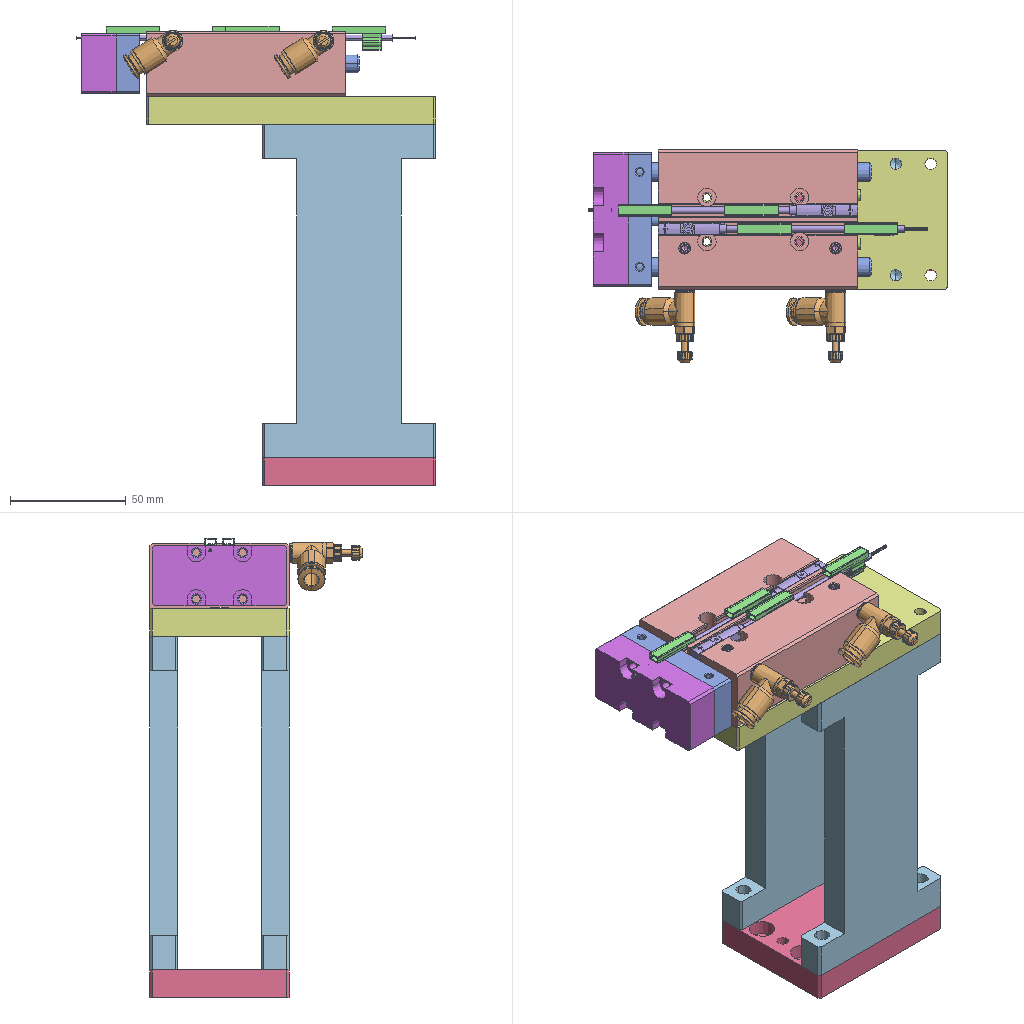Assembly | SolidWorks | 14 different items | 26 placed | box 155 x 91 x 198 mm
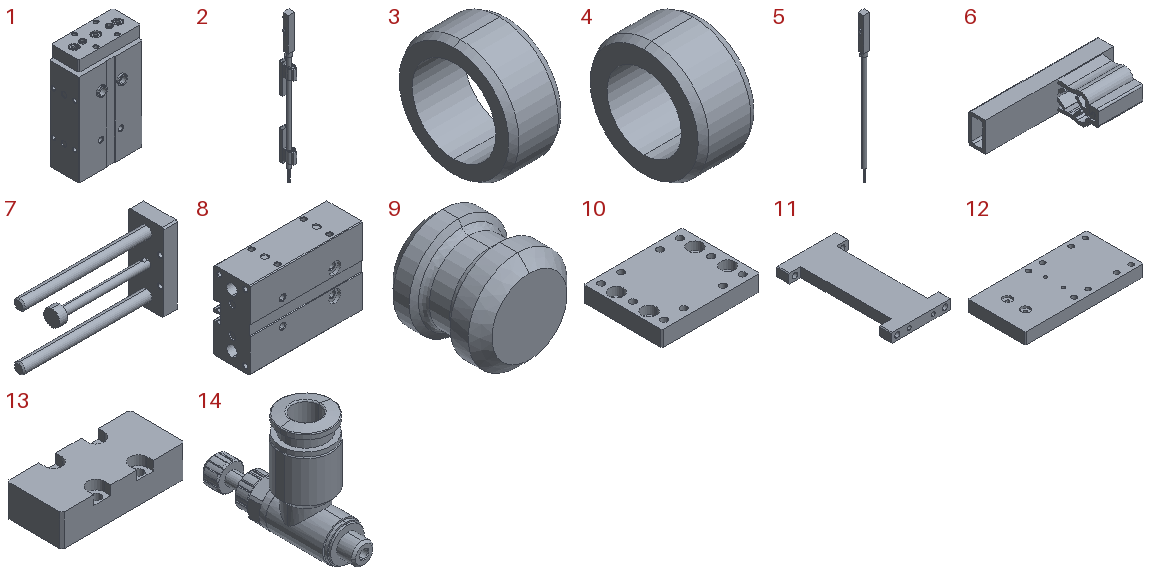Parts list (item | name | quantity | parent item | size | volume | features):
1 | (subassembly) | x1 | - | 60 x 29.95 x 106.2 mm | 146191 mm3 | -
2 | (subassembly) | x2 | - | 6.45 x 10.3 x 116.3 mm | 1707 mm3 | -
3 | - | x2 | in 1 | 4 x 9 x 9 mm | 121.796 mm3 | features BaseBody 1
4 | - | x4 | in 1 | 2.4 x 5 x 5 mm | 27.025 mm3 | features BaseBody 1
5 | - | x2 | in 2 | 6.45 x 4.8 x 116.3 mm | 1119 mm3 | features BaseBody 1
6 | - | x4 | in 2 | 23 x 10.3 x 5.4 mm | 293.788 mm3 | features BaseBody 1
7 | - | x1 | in 1 | 105 x 26 x 58 mm | 26314 mm3 | features BaseBody 1
8 | - | x1 | in 1 | 86 x 28.05 x 60 mm | 119405 mm3 | features BaseBody 1
9 | - | x2 | in 1 | 5 x 5 x 5 mm | 60.215 mm3 | features BaseBody 1
10 | - | x1 | - | 75 x 60 x 12 mm | 48559 mm3 | features HoleWzd 4, Chamfer 1, Extrusion 1
11 | - | x2 | - | 75 x 144 x 12 mm | 85544 mm3 | features HoleWzd 2, MirrorPattern 2, Chamfer 1, Extrusion 1, ICE 1
12 | - | x1 | - | 125 x 60 x 12 mm | 87460 mm3 | features HoleWzd 3, Chamfer 1, Cut 1, Extrusion 1
13 | - | x1 | - | 58 x 26 x 15 mm | 20953 mm3 | features HoleWzd 2, Chamfer 1, Extrusion 1, ICE 1, MirrorPattern 1
14 | - | x2 | - | 11.8 x 35.4 x 26.45 mm | 2728 mm3 | features BaseBody 1
Mates (type | each side: item.copy, entity, surface, feature):
Coincident | 10.1 face plane Boss-Extrude1 | 11.1 face plane Boss-Extrude1
Width | 11.1 face plane Boss-Extrude1 | 11.1 face plane Boss-Extrude1 | 10.1 face plane Boss-Extrude1 | 10.1 face plane Boss-Extrude1
DistanceDim | 11.1 face plane Boss-Extrude1 | 10.1 face plane Boss-Extrude1
Coincident | 10.1 face plane Boss-Extrude1 | 11.2 face plane Boss-Extrude1
Width | 11.2 face plane Boss-Extrude1 | 11.2 face plane Boss-Extrude1 | 10.1 face plane Boss-Extrude1 | 10.1 face plane Boss-Extrude1
Width | 11.2 face plane Boss-Extrude1 | 11.1 face plane Boss-Extrude1 | 10.1 face plane Boss-Extrude1 | 10.1 face plane Boss-Extrude1
Coincident | 11.1 face plane Boss-Extrude1 | 12.1 face plane Boss-Extrude1
Coincident | 11.2 face plane Boss-Extrude1 | 12.1 face plane Boss-Extrude1
Width | 12.1 face plane Boss-Extrude1 | 12.1 face plane Boss-Extrude1 | 11.1 face plane Boss-Extrude1 | 11.2 face plane Boss-Extrude1
Coincident | 12.1 face plane Boss-Extrude1 | 8.1 face plane Input1 | 2 times
Width | 8.1 face plane Input1 | 8.1 face plane Input1 | 12.1 face plane Boss-Extrude1 | 12.1 face plane Boss-Extrude1
Coincident | 7.1 face plane Input1 | 13.1 face plane Boss-Extrude1
Width | 13.1 face plane Boss-Extrude1 | 13.1 face plane Boss-Extrude1 | 7.1 face plane Input1 | 7.1 face plane Input1
Width | 7.1 face plane Input1 | 7.1 face plane Input1 | 13.1 face plane Boss-Extrude1 | 13.1 face plane Boss-Extrude1
Concentric | 8.1 face cylinder Input1 | 14.1 face cylinder Input1
Coincident | 8.1 face plane Input1 | 14.1 face plane Input1
Concentric | 8.1 face cylinder Input1 | 14.2 face cylinder Input1
Coincident | 8.1 face plane Input1 | 14.2 face plane Input1
Width | 5.1 face plane Input1 | 5.1 face plane Input1 | 8.1 face plane Input1 | 8.1 face plane Input1
Coincident | 8.1 face plane Input1 | 5.1 face plane Input1 | 2 times
Width | 8.1 face plane Input1 | 8.1 face plane Input1 | 5.2 face plane Input1 | 5.2 face plane Input1
Coincident | 8.1 face plane Input1 | 5.2 face plane Input1 | 2 times